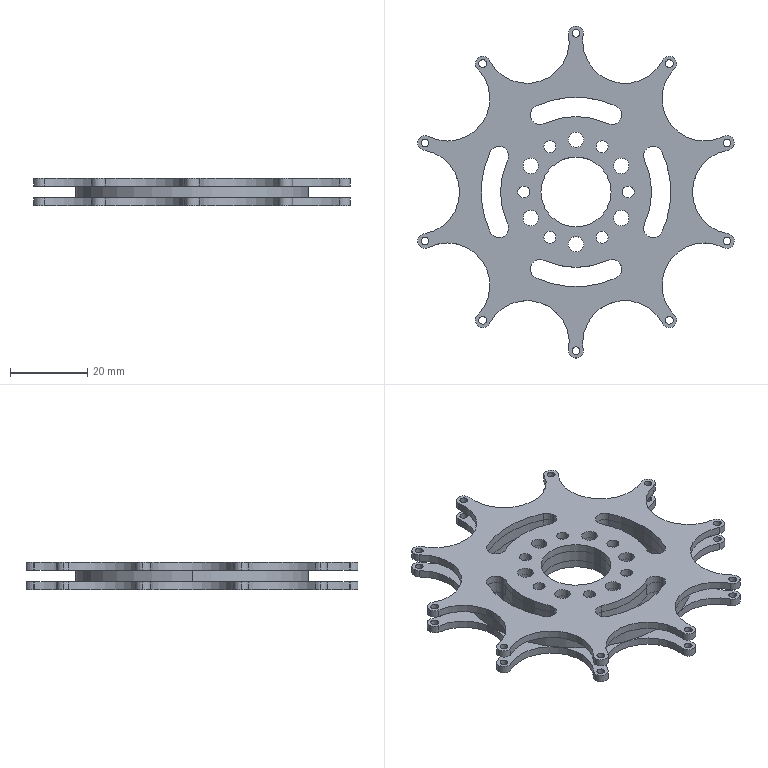Part | SolidWorks | features ICE 4, Extrusion 1 | 3 solids | 258 faces | box 81.787 x 85.8 x 7 mm | volume 16789 mm3 | cylinder 252 | plane 6 | commonest cylinder face diameters 2 x40 3.1 x36 3.8 x36 4 x36 5 x36 21.855 x30